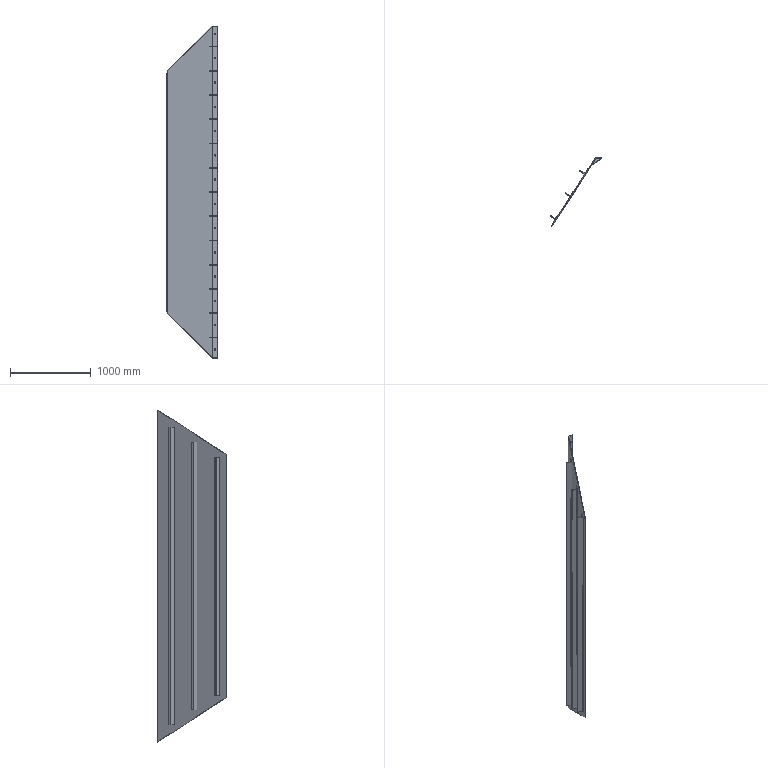Part | STEP file | Side plate assembly 2_Default<As machined> | 17 solids | 149 faces | box 630.687 x 850.025 x 4105 mm | volume 42475037 mm3 | plane 97 | cylinder 52 | commonest cylinder face diameters 18 x31 4 x14 5.333 x6 20 x1